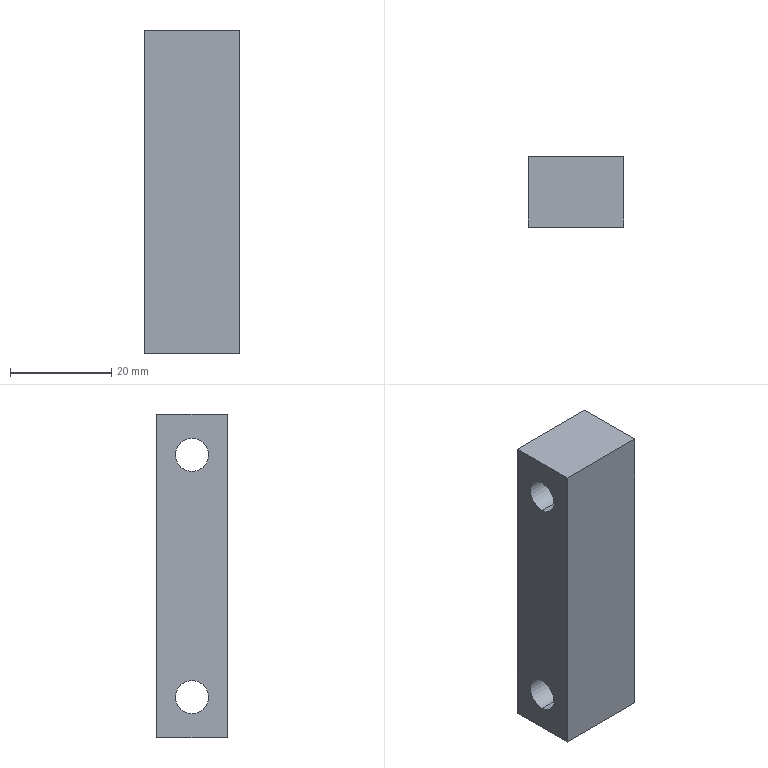Part | STEP file | 1 solid | 16 faces | box 19 x 14 x 64 mm | volume 14945 mm3 | cylinder 8 | plane 8 | commonest cylinder face diameters 6.6 x4 11 x4
STEP:
#1=CARTESIAN_POINT('',(0.,0.,0.));
#2=DIRECTION('',(0.,0.,1.));
#3=DIRECTION('',(1.,0.,0.));
#4=AXIS2_PLACEMENT_3D('',#1,#2,#3);
#5=CARTESIAN_POINT('',(12.6,0.,18.5));
#6=VERTEX_POINT('',#5);
#7=CARTESIAN_POINT('',(19.,0.,18.5));
#8=VERTEX_POINT('',#7);
#9=CARTESIAN_POINT('',(19.,0.,18.5));
#10=DIRECTION('',(1.,0.,0.));
#11=VECTOR('',#10,1.);
#12=LINE('',#9,#11);
#13=CARTESIAN_POINT('',(19.,0.,24.));
#14=DIRECTION('',(1.,0.,0.));
#15=DIRECTION('',(0.,0.,-1.));
#16=AXIS2_PLACEMENT_3D('',#13,#14,#15);
#17=CYLINDRICAL_SURFACE('',#16,5.5);
#18=CARTESIAN_POINT('',(6.283,0.));
#19=DIRECTION('',(0.,1.));
#20=VECTOR('',#19,1.);
#21=LINE('',#18,#20);
#22=(GEOMETRIC_REPRESENTATION_CONTEXT(2)PARAMETRIC_REPRESENTATION_CONTEXT()REPRESENTATION_CONTEXT('',''));
#23=DEFINITIONAL_REPRESENTATION('',(#21),#22);
#24=PCURVE('',#17,#23);
#25=CARTESIAN_POINT('',(19.,0.,24.));
#26=DIRECTION('',(1.,0.,0.));
#27=DIRECTION('',(0.,0.,-1.));
#28=AXIS2_PLACEMENT_3D('',#25,#26,#27);
#29=CYLINDRICAL_SURFACE('',#28,5.5);
#30=CARTESIAN_POINT('',(0.,0.));
#31=DIRECTION('',(0.,1.));
#32=VECTOR('',#31,1.);
#33=LINE('',#30,#32);
#34=(GEOMETRIC_REPRESENTATION_CONTEXT(2)PARAMETRIC_REPRESENTATION_CONTEXT()REPRESENTATION_CONTEXT('',''));
#35=DEFINITIONAL_REPRESENTATION('',(#33),#34);
#36=PCURVE('',#29,#35);
#37=SURFACE_CURVE('',#12,(#24,#36),.PCURVE_S1.);
#38=EDGE_CURVE('',#6,#8,#37,.T.);
#39=ORIENTED_EDGE('',*,*,#38,.T.);
#40=CARTESIAN_POINT('',(19.,0.,29.5));
#41=VERTEX_POINT('',#40);
#42=CARTESIAN_POINT('',(19.,0.,24.));
#43=DIRECTION('',(1.,0.,0.));
#44=DIRECTION('',(0.,0.,-1.));
#45=AXIS2_PLACEMENT_3D('',#42,#43,#44);
#46=CIRCLE('',#45,5.5);
#47=CARTESIAN_POINT('',(0.,0.));
#48=DIRECTION('',(1.,0.));
#49=VECTOR('',#48,1.);
#50=LINE('',#47,#49);
#51=(GEOMETRIC_REPRESENTATION_CONTEXT(2)PARAMETRIC_REPRESENTATION_CONTEXT()REPRESENTATION_CONTEXT('',''));
#52=DEFINITIONAL_REPRESENTATION('',(#50),#51);
#53=PCURVE('',#17,#52);
#54=CARTESIAN_POINT('',(19.,0.,0.));
#55=DIRECTION('',(1.,0.,0.));
#56=DIRECTION('',(0.,0.,-1.));
#57=AXIS2_PLACEMENT_3D('',#54,#55,#56);
#58=PLANE('',#57);
#59=CARTESIAN_POINT('',(-24.,0.));
#60=DIRECTION('',(1.,0.));
#61=AXIS2_PLACEMENT_2D('',#59,#60);
#62=CIRCLE('',#61,5.5);
#63=(GEOMETRIC_REPRESENTATION_CONTEXT(2)PARAMETRIC_REPRESENTATION_CONTEXT()REPRESENTATION_CONTEXT('',''));
#64=DEFINITIONAL_REPRESENTATION('',(#62),#63);
#65=PCURVE('',#58,#64);
#66=SURFACE_CURVE('',#46,(#53,#65),.PCURVE_S1.);
#67=EDGE_CURVE('',#41,#8,#66,.T.);
#68=ORIENTED_EDGE('',*,*,#67,.F.);
#69=CARTESIAN_POINT('',(12.6,0.,29.5));
#70=VERTEX_POINT('',#69);
#71=CARTESIAN_POINT('',(19.,0.,29.5));
#72=DIRECTION('',(1.,0.,0.));
#73=VECTOR('',#72,1.);
#74=LINE('',#71,#73);
#75=CARTESIAN_POINT('',(3.142,0.));
#76=DIRECTION('',(0.,1.));
#77=VECTOR('',#76,1.);
#78=LINE('',#75,#77);
#79=(GEOMETRIC_REPRESENTATION_CONTEXT(2)PARAMETRIC_REPRESENTATION_CONTEXT()REPRESENTATION_CONTEXT('',''));
#80=DEFINITIONAL_REPRESENTATION('',(#78),#79);
#81=PCURVE('',#17,#80);
#82=CARTESIAN_POINT('',(3.142,0.));
#83=DIRECTION('',(0.,1.));
#84=VECTOR('',#83,1.);
#85=LINE('',#82,#84);
#86=(GEOMETRIC_REPRESENTATION_CONTEXT(2)PARAMETRIC_REPRESENTATION_CONTEXT()REPRESENTATION_CONTEXT('',''));
#87=DEFINITIONAL_REPRESENTATION('',(#85),#86);
#88=PCURVE('',#29,#87);
#89=SURFACE_CURVE('',#74,(#81,#88),.PCURVE_S1.);
#90=EDGE_CURVE('',#70,#41,#89,.T.);
#91=ORIENTED_EDGE('',*,*,#90,.F.);
#92=CARTESIAN_POINT('',(12.6,0.,24.));
#93=DIRECTION('',(1.,0.,0.));
#94=DIRECTION('',(0.,0.,-1.));
#95=AXIS2_PLACEMENT_3D('',#92,#93,#94);
#96=CIRCLE('',#95,5.5);
#97=CARTESIAN_POINT('',(0.,-6.4));
#98=DIRECTION('',(1.,0.));
#99=VECTOR('',#98,1.);
#100=LINE('',#97,#99);
#101=(GEOMETRIC_REPRESENTATION_CONTEXT(2)PARAMETRIC_REPRESENTATION_CONTEXT()REPRESENTATION_CONTEXT('',''));
#102=DEFINITIONAL_REPRESENTATION('',(#100),#101);
#103=PCURVE('',#17,#102);
#104=CARTESIAN_POINT('',(12.6,3.3,24.));
#105=DIRECTION('',(-1.,0.,0.));
#106=DIRECTION('',(0.,0.,1.));
#107=AXIS2_PLACEMENT_3D('',#104,#105,#106);
#108=PLANE('',#107);
#109=CARTESIAN_POINT('',(-5.5,-3.3));
#110=CARTESIAN_POINT('',(-5.5,6.226));
#111=CARTESIAN_POINT('',(2.75,1.463));
#112=CARTESIAN_POINT('',(11.,-3.3));
#113=CARTESIAN_POINT('',(2.75,-8.063));
#114=CARTESIAN_POINT('',(-5.5,-12.826));
#115=CARTESIAN_POINT('',(-5.5,-3.3));
#116=(BOUNDED_CURVE()B_SPLINE_CURVE(2,(#109,#110,#111,#112,#113,#114,#115),.UNSPECIFIED.,.T.,.F.)B_SPLINE_CURVE_WITH_KNOTS((1,2,2,2,2,1),(-2.094,0.,2.094,4.189,6.283,8.378),.UNSPECIFIED.)CURVE()GEOMETRIC_REPRESENTATION_ITEM()RATIONAL_B_SPLINE_CURVE((1.,0.5,1.,0.5,1.,0.5,1.))REPRESENTATION_ITEM(''));
#117=(GEOMETRIC_REPRESENTATION_CONTEXT(2)PARAMETRIC_REPRESENTATION_CONTEXT()REPRESENTATION_CONTEXT('',''));
#118=DEFINITIONAL_REPRESENTATION('',(#116),#117);
#119=PCURVE('',#108,#118);
#120=SURFACE_CURVE('',#96,(#103,#119),.PCURVE_S1.);
#121=EDGE_CURVE('',#70,#6,#120,.T.);
#122=ORIENTED_EDGE('',*,*,#121,.T.);
#123=EDGE_LOOP('',(#39,#68,#91,#122));
#124=FACE_BOUND('',#123,.F.);
#125=ADVANCED_FACE('',(#124),#17,.F.);
#126=CARTESIAN_POINT('',(0.,0.,20.7));
#127=VERTEX_POINT('',#126);
#128=CARTESIAN_POINT('',(12.6,0.,20.7));
#129=VERTEX_POINT('',#128);
#130=CARTESIAN_POINT('',(19.,0.,20.7));
#131=DIRECTION('',(1.,0.,0.));
#132=VECTOR('',#131,1.);
#133=LINE('',#130,#132);
#134=CARTESIAN_POINT('',(19.,0.,24.));
#135=DIRECTION('',(1.,0.,0.));
#136=DIRECTION('',(0.,0.,-1.));
#137=AXIS2_PLACEMENT_3D('',#134,#135,#136);
#138=CYLINDRICAL_SURFACE('',#137,3.3);
#139=CARTESIAN_POINT('',(6.283,0.));
#140=DIRECTION('',(0.,1.));
#141=VECTOR('',#140,1.);
#142=LINE('',#139,#141);
#143=(GEOMETRIC_REPRESENTATION_CONTEXT(2)PARAMETRIC_REPRESENTATION_CONTEXT()REPRESENTATION_CONTEXT('',''));
#144=DEFINITIONAL_REPRESENTATION('',(#142),#143);
#145=PCURVE('',#138,#144);
#146=CARTESIAN_POINT('',(19.,0.,24.));
#147=DIRECTION('',(1.,0.,0.));
#148=DIRECTION('',(0.,0.,-1.));
#149=AXIS2_PLACEMENT_3D('',#146,#147,#148);
#150=CYLINDRICAL_SURFACE('',#149,3.3);
#151=CARTESIAN_POINT('',(0.,0.));
#152=DIRECTION('',(0.,1.));
#153=VECTOR('',#152,1.);
#154=LINE('',#151,#153);
#155=(GEOMETRIC_REPRESENTATION_CONTEXT(2)PARAMETRIC_REPRESENTATION_CONTEXT()REPRESENTATION_CONTEXT('',''));
#156=DEFINITIONAL_REPRESENTATION('',(#154),#155);
#157=PCURVE('',#150,#156);
#158=SURFACE_CURVE('',#133,(#145,#157),.PCURVE_S1.);
#159=EDGE_CURVE('',#127,#129,#158,.T.);
#160=ORIENTED_EDGE('',*,*,#159,.T.);
#161=CARTESIAN_POINT('',(12.6,0.,27.3));
#162=VERTEX_POINT('',#161);
#163=CARTESIAN_POINT('',(12.6,0.,24.));
#164=DIRECTION('',(1.,0.,0.));
#165=DIRECTION('',(0.,0.,-1.));
#166=AXIS2_PLACEMENT_3D('',#163,#164,#165);
#167=CIRCLE('',#166,3.3);
#168=CARTESIAN_POINT('',(0.,-6.4));
#169=DIRECTION('',(1.,0.));
#170=VECTOR('',#169,1.);
#171=LINE('',#168,#170);
#172=(GEOMETRIC_REPRESENTATION_CONTEXT(2)PARAMETRIC_REPRESENTATION_CONTEXT()REPRESENTATION_CONTEXT('',''));
#173=DEFINITIONAL_REPRESENTATION('',(#171),#172);
#174=PCURVE('',#138,#173);
#175=CARTESIAN_POINT('',(-3.3,-3.3));
#176=CARTESIAN_POINT('',(-3.3,2.416));
#177=CARTESIAN_POINT('',(1.65,-0.4421));
#178=CARTESIAN_POINT('',(6.6,-3.3));
#179=CARTESIAN_POINT('',(1.65,-6.158));
#180=CARTESIAN_POINT('',(-3.3,-9.016));
#181=CARTESIAN_POINT('',(-3.3,-3.3));
#182=(BOUNDED_CURVE()B_SPLINE_CURVE(2,(#175,#176,#177,#178,#179,#180,#181),.UNSPECIFIED.,.T.,.F.)B_SPLINE_CURVE_WITH_KNOTS((1,2,2,2,2,1),(-2.094,0.,2.094,4.189,6.283,8.378),.UNSPECIFIED.)CURVE()GEOMETRIC_REPRESENTATION_ITEM()RATIONAL_B_SPLINE_CURVE((1.,0.5,1.,0.5,1.,0.5,1.))REPRESENTATION_ITEM(''));
#183=(GEOMETRIC_REPRESENTATION_CONTEXT(2)PARAMETRIC_REPRESENTATION_CONTEXT()REPRESENTATION_CONTEXT('',''));
#184=DEFINITIONAL_REPRESENTATION('',(#182),#183);
#185=PCURVE('',#108,#184);
#186=SURFACE_CURVE('',#167,(#174,#185),.PCURVE_S1.);
#187=EDGE_CURVE('',#162,#129,#186,.T.);
#188=ORIENTED_EDGE('',*,*,#187,.F.);
#189=CARTESIAN_POINT('',(0.,0.,27.3));
#190=VERTEX_POINT('',#189);
#191=CARTESIAN_POINT('',(19.,0.,27.3));
#192=DIRECTION('',(1.,0.,0.));
#193=VECTOR('',#192,1.);
#194=LINE('',#191,#193);
#195=CARTESIAN_POINT('',(3.142,0.));
#196=DIRECTION('',(0.,1.));
#197=VECTOR('',#196,1.);
#198=LINE('',#195,#197);
#199=(GEOMETRIC_REPRESENTATION_CONTEXT(2)PARAMETRIC_REPRESENTATION_CONTEXT()REPRESENTATION_CONTEXT('',''));
#200=DEFINITIONAL_REPRESENTATION('',(#198),#199);
#201=PCURVE('',#138,#200);
#202=CARTESIAN_POINT('',(3.142,0.));
#203=DIRECTION('',(0.,1.));
#204=VECTOR('',#203,1.);
#205=LINE('',#202,#204);
#206=(GEOMETRIC_REPRESENTATION_CONTEXT(2)PARAMETRIC_REPRESENTATION_CONTEXT()REPRESENTATION_CONTEXT('',''));
#207=DEFINITIONAL_REPRESENTATION('',(#205),#206);
#208=PCURVE('',#150,#207);
#209=SURFACE_CURVE('',#194,(#201,#208),.PCURVE_S1.);
#210=EDGE_CURVE('',#190,#162,#209,.T.);
#211=ORIENTED_EDGE('',*,*,#210,.F.);
#212=CARTESIAN_POINT('',(0.,0.,24.));
#213=DIRECTION('',(1.,0.,0.));
#214=DIRECTION('',(0.,0.,-1.));
#215=AXIS2_PLACEMENT_3D('',#212,#213,#214);
#216=CIRCLE('',#215,3.3);
#217=CARTESIAN_POINT('',(0.,-19.));
#218=DIRECTION('',(1.,0.));
#219=VECTOR('',#218,1.);
#220=LINE('',#217,#219);
#221=(GEOMETRIC_REPRESENTATION_CONTEXT(2)PARAMETRIC_REPRESENTATION_CONTEXT()REPRESENTATION_CONTEXT('',''));
#222=DEFINITIONAL_REPRESENTATION('',(#220),#221);
#223=PCURVE('',#138,#222);
#224=CARTESIAN_POINT('',(0.,0.,0.));
#225=DIRECTION('',(1.,0.,0.));
#226=DIRECTION('',(0.,0.,-1.));
#227=AXIS2_PLACEMENT_3D('',#224,#225,#226);
#228=PLANE('',#227);
#229=CARTESIAN_POINT('',(-24.,0.));
#230=DIRECTION('',(1.,0.));
#231=AXIS2_PLACEMENT_2D('',#229,#230);
#232=CIRCLE('',#231,3.3);
#233=(GEOMETRIC_REPRESENTATION_CONTEXT(2)PARAMETRIC_REPRESENTATION_CONTEXT()REPRESENTATION_CONTEXT('',''));
#234=DEFINITIONAL_REPRESENTATION('',(#232),#233);
#235=PCURVE('',#228,#234);
#236=SURFACE_CURVE('',#216,(#223,#235),.PCURVE_S1.);
#237=EDGE_CURVE('',#190,#127,#236,.T.);
#238=ORIENTED_EDGE('',*,*,#237,.T.);
#239=EDGE_LOOP('',(#160,#188,#211,#238));
#240=FACE_BOUND('',#239,.F.);
#241=ADVANCED_FACE('',(#240),#138,.F.);
#242=CARTESIAN_POINT('',(12.6,0.,-29.5));
#243=VERTEX_POINT('',#242);
#244=CARTESIAN_POINT('',(19.,0.,-29.5));
#245=VERTEX_POINT('',#244);
#246=CARTESIAN_POINT('',(19.,0.,-29.5));
#247=DIRECTION('',(1.,0.,0.));
#248=VECTOR('',#247,1.);
#249=LINE('',#246,#248);
#250=CARTESIAN_POINT('',(19.,0.,-24.));
#251=DIRECTION('',(1.,0.,0.));
#252=DIRECTION('',(0.,0.,-1.));
#253=AXIS2_PLACEMENT_3D('',#250,#251,#252);
#254=CYLINDRICAL_SURFACE('',#253,5.5);
#255=CARTESIAN_POINT('',(6.283,0.));
#256=DIRECTION('',(0.,1.));
#257=VECTOR('',#256,1.);
#258=LINE('',#255,#257);
#259=(GEOMETRIC_REPRESENTATION_CONTEXT(2)PARAMETRIC_REPRESENTATION_CONTEXT()REPRESENTATION_CONTEXT('',''));
#260=DEFINITIONAL_REPRESENTATION('',(#258),#259);
#261=PCURVE('',#254,#260);
#262=CARTESIAN_POINT('',(19.,0.,-24.));
#263=DIRECTION('',(1.,0.,0.));
#264=DIRECTION('',(0.,0.,-1.));
#265=AXIS2_PLACEMENT_3D('',#262,#263,#264);
#266=CYLINDRICAL_SURFACE('',#265,5.5);
#267=CARTESIAN_POINT('',(0.,0.));
#268=DIRECTION('',(0.,1.));
#269=VECTOR('',#268,1.);
#270=LINE('',#267,#269);
#271=(GEOMETRIC_REPRESENTATION_CONTEXT(2)PARAMETRIC_REPRESENTATION_CONTEXT()REPRESENTATION_CONTEXT('',''));
#272=DEFINITIONAL_REPRESENTATION('',(#270),#271);
#273=PCURVE('',#266,#272);
#274=SURFACE_CURVE('',#249,(#261,#273),.PCURVE_S1.);
#275=EDGE_CURVE('',#243,#245,#274,.T.);
#276=ORIENTED_EDGE('',*,*,#275,.T.);
#277=CARTESIAN_POINT('',(19.,0.,-18.5));
#278=VERTEX_POINT('',#277);
#279=CARTESIAN_POINT('',(19.,0.,-24.));
#280=DIRECTION('',(1.,0.,0.));
#281=DIRECTION('',(0.,0.,-1.));
#282=AXIS2_PLACEMENT_3D('',#279,#280,#281);
#283=CIRCLE('',#282,5.5);
#284=CARTESIAN_POINT('',(0.,0.));
#285=DIRECTION('',(1.,0.));
#286=VECTOR('',#285,1.);
#287=LINE('',#284,#286);
#288=(GEOMETRIC_REPRESENTATION_CONTEXT(2)PARAMETRIC_REPRESENTATION_CONTEXT()REPRESENTATION_CONTEXT('',''));
#289=DEFINITIONAL_REPRESENTATION('',(#287),#288);
#290=PCURVE('',#254,#289);
#291=CARTESIAN_POINT('',(24.,0.));
#292=DIRECTION('',(1.,0.));
#293=AXIS2_PLACEMENT_2D('',#291,#292);
#294=CIRCLE('',#293,5.5);
#295=(GEOMETRIC_REPRESENTATION_CONTEXT(2)PARAMETRIC_REPRESENTATION_CONTEXT()REPRESENTATION_CONTEXT('',''));
#296=DEFINITIONAL_REPRESENTATION('',(#294),#295);
#297=PCURVE('',#58,#296);
#298=SURFACE_CURVE('',#283,(#290,#297),.PCURVE_S1.);
#299=EDGE_CURVE('',#278,#245,#298,.T.);
#300=ORIENTED_EDGE('',*,*,#299,.F.);
#301=CARTESIAN_POINT('',(12.6,0.,-18.5));
#302=VERTEX_POINT('',#301);
#303=CARTESIAN_POINT('',(19.,0.,-18.5));
#304=DIRECTION('',(1.,0.,0.));
#305=VECTOR('',#304,1.);
#306=LINE('',#303,#305);
#307=CARTESIAN_POINT('',(3.142,0.));
#308=DIRECTION('',(0.,1.));
#309=VECTOR('',#308,1.);
#310=LINE('',#307,#309);
#311=(GEOMETRIC_REPRESENTATION_CONTEXT(2)PARAMETRIC_REPRESENTATION_CONTEXT()REPRESENTATION_CONTEXT('',''));
#312=DEFINITIONAL_REPRESENTATION('',(#310),#311);
#313=PCURVE('',#254,#312);
#314=CARTESIAN_POINT('',(3.142,0.));
#315=DIRECTION('',(0.,1.));
#316=VECTOR('',#315,1.);
#317=LINE('',#314,#316);
#318=(GEOMETRIC_REPRESENTATION_CONTEXT(2)PARAMETRIC_REPRESENTATION_CONTEXT()REPRESENTATION_CONTEXT('',''));
#319=DEFINITIONAL_REPRESENTATION('',(#317),#318);
#320=PCURVE('',#266,#319);
#321=SURFACE_CURVE('',#306,(#313,#320),.PCURVE_S1.);
#322=EDGE_CURVE('',#302,#278,#321,.T.);
#323=ORIENTED_EDGE('',*,*,#322,.F.);
#324=CARTESIAN_POINT('',(12.6,0.,-24.));
#325=DIRECTION('',(1.,0.,0.));
#326=DIRECTION('',(0.,0.,-1.));
#327=AXIS2_PLACEMENT_3D('',#324,#325,#326);
#328=CIRCLE('',#327,5.5);
#329=CARTESIAN_POINT('',(0.,-6.4));
#330=DIRECTION('',(1.,0.));
#331=VECTOR('',#330,1.);
#332=LINE('',#329,#331);
#333=(GEOMETRIC_REPRESENTATION_CONTEXT(2)PARAMETRIC_REPRESENTATION_CONTEXT()REPRESENTATION_CONTEXT('',''));
#334=DEFINITIONAL_REPRESENTATION('',(#332),#333);
#335=PCURVE('',#254,#334);
#336=CARTESIAN_POINT('',(12.6,3.3,-24.));
#337=DIRECTION('',(-1.,0.,0.));
#338=DIRECTION('',(0.,0.,1.));
#339=AXIS2_PLACEMENT_3D('',#336,#337,#338);
#340=PLANE('',#339);
#341=CARTESIAN_POINT('',(-5.5,-3.3));
#342=CARTESIAN_POINT('',(-5.5,6.226));
#343=CARTESIAN_POINT('',(2.75,1.463));
#344=CARTESIAN_POINT('',(11.,-3.3));
#345=CARTESIAN_POINT('',(2.75,-8.063));
#346=CARTESIAN_POINT('',(-5.5,-12.826));
#347=CARTESIAN_POINT('',(-5.5,-3.3));
#348=(BOUNDED_CURVE()B_SPLINE_CURVE(2,(#341,#342,#343,#344,#345,#346,#347),.UNSPECIFIED.,.T.,.F.)B_SPLINE_CURVE_WITH_KNOTS((1,2,2,2,2,1),(-2.094,0.,2.094,4.189,6.283,8.378),.UNSPECIFIED.)CURVE()GEOMETRIC_REPRESENTATION_ITEM()RATIONAL_B_SPLINE_CURVE((1.,0.5,1.,0.5,1.,0.5,1.))REPRESENTATION_ITEM(''));
#349=(GEOMETRIC_REPRESENTATION_CONTEXT(2)PARAMETRIC_REPRESENTATION_CONTEXT()REPRESENTATION_CONTEXT('',''));
#350=DEFINITIONAL_REPRESENTATION('',(#348),#349);
#351=PCURVE('',#340,#350);
#352=SURFACE_CURVE('',#328,(#335,#351),.PCURVE_S1.);
#353=EDGE_CURVE('',#302,#243,#352,.T.);
#354=ORIENTED_EDGE('',*,*,#353,.T.);
#355=EDGE_LOOP('',(#276,#300,#323,#354));
#356=FACE_BOUND('',#355,.F.);
#357=ADVANCED_FACE('',(#356),#254,.F.);
#358=CARTESIAN_POINT('',(0.,0.,-27.3));
#359=VERTEX_POINT('',#358);
#360=CARTESIAN_POINT('',(12.6,0.,-27.3));
#361=VERTEX_POINT('',#360);
#362=CARTESIAN_POINT('',(19.,0.,-27.3));
#363=DIRECTION('',(1.,0.,0.));
#364=VECTOR('',#363,1.);
#365=LINE('',#362,#364);
#366=CARTESIAN_POINT('',(19.,0.,-24.));
#367=DIRECTION('',(1.,0.,0.));
#368=DIRECTION('',(0.,0.,-1.));
#369=AXIS2_PLACEMENT_3D('',#366,#367,#368);
#370=CYLINDRICAL_SURFACE('',#369,3.3);
#371=CARTESIAN_POINT('',(6.283,0.));
#372=DIRECTION('',(0.,1.));
#373=VECTOR('',#372,1.);
#374=LINE('',#371,#373);
#375=(GEOMETRIC_REPRESENTATION_CONTEXT(2)PARAMETRIC_REPRESENTATION_CONTEXT()REPRESENTATION_CONTEXT('',''));
#376=DEFINITIONAL_REPRESENTATION('',(#374),#375);
#377=PCURVE('',#370,#376);
#378=CARTESIAN_POINT('',(19.,0.,-24.));
#379=DIRECTION('',(1.,0.,0.));
#380=DIRECTION('',(0.,0.,-1.));
#381=AXIS2_PLACEMENT_3D('',#378,#379,#380);
#382=CYLINDRICAL_SURFACE('',#381,3.3);
#383=CARTESIAN_POINT('',(0.,0.));
#384=DIRECTION('',(0.,1.));
#385=VECTOR('',#384,1.);
#386=LINE('',#383,#385);
#387=(GEOMETRIC_REPRESENTATION_CONTEXT(2)PARAMETRIC_REPRESENTATION_CONTEXT()REPRESENTATION_CONTEXT('',''));
#388=DEFINITIONAL_REPRESENTATION('',(#386),#387);
#389=PCURVE('',#382,#388);
#390=SURFACE_CURVE('',#365,(#377,#389),.PCURVE_S1.);
#391=EDGE_CURVE('',#359,#361,#390,.T.);
#392=ORIENTED_EDGE('',*,*,#391,.T.);
#393=CARTESIAN_POINT('',(12.6,0.,-20.7));
#394=VERTEX_POINT('',#393);
#395=CARTESIAN_POINT('',(12.6,0.,-24.));
#396=DIRECTION('',(1.,0.,0.));
#397=DIRECTION('',(0.,0.,-1.));
#398=AXIS2_PLACEMENT_3D('',#395,#396,#397);
#399=CIRCLE('',#398,3.3);
#400=CARTESIAN_POINT('',(0.,-6.4));
#401=DIRECTION('',(1.,0.));
#402=VECTOR('',#401,1.);
#403=LINE('',#400,#402);
#404=(GEOMETRIC_REPRESENTATION_CONTEXT(2)PARAMETRIC_REPRESENTATION_CONTEXT()REPRESENTATION_CONTEXT('',''));
#405=DEFINITIONAL_REPRESENTATION('',(#403),#404);
#406=PCURVE('',#370,#405);
#407=CARTESIAN_POINT('',(-3.3,-3.3));
#408=CARTESIAN_POINT('',(-3.3,2.416));
#409=CARTESIAN_POINT('',(1.65,-0.4421));
#410=CARTESIAN_POINT('',(6.6,-3.3));
#411=CARTESIAN_POINT('',(1.65,-6.158));
#412=CARTESIAN_POINT('',(-3.3,-9.016));
#413=CARTESIAN_POINT('',(-3.3,-3.3));
#414=(BOUNDED_CURVE()B_SPLINE_CURVE(2,(#407,#408,#409,#410,#411,#412,#413),.UNSPECIFIED.,.T.,.F.)B_SPLINE_CURVE_WITH_KNOTS((1,2,2,2,2,1),(-2.094,0.,2.094,4.189,6.283,8.378),.UNSPECIFIED.)CURVE()GEOMETRIC_REPRESENTATION_ITEM()RATIONAL_B_SPLINE_CURVE((1.,0.5,1.,0.5,1.,0.5,1.))REPRESENTATION_ITEM(''));
#415=(GEOMETRIC_REPRESENTATION_CONTEXT(2)PARAMETRIC_REPRESENTATION_CONTEXT()REPRESENTATION_CONTEXT('',''));
#416=DEFINITIONAL_REPRESENTATION('',(#414),#415);
#417=PCURVE('',#340,#416);
#418=SURFACE_CURVE('',#399,(#406,#417),.PCURVE_S1.);
#419=EDGE_CURVE('',#394,#361,#418,.T.);
#420=ORIENTED_EDGE('',*,*,#419,.F.);
#421=CARTESIAN_POINT('',(0.,0.,-20.7));
#422=VERTEX_POINT('',#421);
#423=CARTESIAN_POINT('',(19.,0.,-20.7));
#424=DIRECTION('',(1.,0.,0.));
#425=VECTOR('',#424,1.);
#426=LINE('',#423,#425);
#427=CARTESIAN_POINT('',(3.142,0.));
#428=DIRECTION('',(0.,1.));
#429=VECTOR('',#428,1.);
#430=LINE('',#427,#429);
#431=(GEOMETRIC_REPRESENTATION_CONTEXT(2)PARAMETRIC_REPRESENTATION_CONTEXT()REPRESENTATION_CONTEXT('',''));
#432=DEFINITIONAL_REPRESENTATION('',(#430),#431);
#433=PCURVE('',#370,#432);
#434=CARTESIAN_POINT('',(3.142,0.));
#435=DIRECTION('',(0.,1.));
#436=VECTOR('',#435,1.);
#437=LINE('',#434,#436);
#438=(GEOMETRIC_REPRESENTATION_CONTEXT(2)PARAMETRIC_REPRESENTATION_CONTEXT()REPRESENTATION_CONTEXT('',''));
#439=DEFINITIONAL_REPRESENTATION('',(#437),#438);
#440=PCURVE('',#382,#439);
#441=SURFACE_CURVE('',#426,(#433,#440),.PCURVE_S1.);
#442=EDGE_CURVE('',#422,#394,#441,.T.);
#443=ORIENTED_EDGE('',*,*,#442,.F.);
#444=CARTESIAN_POINT('',(0.,0.,-24.));
#445=DIRECTION('',(1.,0.,0.));
#446=DIRECTION('',(0.,0.,-1.));
#447=AXIS2_PLACEMENT_3D('',#444,#445,#446);
#448=CIRCLE('',#447,3.3);
#449=CARTESIAN_POINT('',(0.,-19.));
#450=DIRECTION('',(1.,0.));
#451=VECTOR('',#450,1.);
#452=LINE('',#449,#451);
#453=(GEOMETRIC_REPRESENTATION_CONTEXT(2)PARAMETRIC_REPRESENTATION_CONTEXT()REPRESENTATION_CONTEXT('',''));
#454=DEFINITIONAL_REPRESENTATION('',(#452),#453);
#455=PCURVE('',#370,#454);
#456=CARTESIAN_POINT('',(24.,0.));
#457=DIRECTION('',(1.,0.));
#458=AXIS2_PLACEMENT_2D('',#456,#457);
#459=CIRCLE('',#458,3.3);
#460=(GEOMETRIC_REPRESENTATION_CONTEXT(2)PARAMETRIC_REPRESENTATION_CONTEXT()REPRESENTATION_CONTEXT('',''));
#461=DEFINITIONAL_REPRESENTATION('',(#459),#460);
#462=PCURVE('',#228,#461);
#463=SURFACE_CURVE('',#448,(#455,#462),.PCURVE_S1.);
#464=EDGE_CURVE('',#422,#359,#463,.T.);
#465=ORIENTED_EDGE('',*,*,#464,.T.);
#466=EDGE_LOOP('',(#392,#420,#443,#465));
#467=FACE_BOUND('',#466,.F.);
#468=ADVANCED_FACE('',(#467),#370,.F.);
#469=CARTESIAN_POINT('',(0.,7.,32.));
#470=VERTEX_POINT('',#469);
#471=CARTESIAN_POINT('',(0.,-7.,32.));
#472=VERTEX_POINT('',#471);
#473=CARTESIAN_POINT('',(0.,-7.,32.));
#474=DIRECTION('',(0.,-1.,0.));
#475=VECTOR('',#474,1.);
#476=LINE('',#473,#475);
#477=CARTESIAN_POINT('',(19.,-7.,32.));
#478=DIRECTION('',(0.,0.,-1.));
#479=DIRECTION('',(-1.,0.,0.));
#480=AXIS2_PLACEMENT_3D('',#477,#478,#479);
#481=PLANE('',#480);
#482=CARTESIAN_POINT('',(19.,0.));
#483=DIRECTION('',(0.,-1.));
#484=VECTOR('',#483,1.);
#485=LINE('',#482,#484);
#486=(GEOMETRIC_REPRESENTATION_CONTEXT(2)PARAMETRIC_REPRESENTATION_CONTEXT()REPRESENTATION_CONTEXT('',''));
#487=DEFINITIONAL_REPRESENTATION('',(#485),#486);
#488=PCURVE('',#481,#487);
#489=CARTESIAN_POINT('',(-32.,-7.));
#490=DIRECTION('',(0.,-1.));
#491=VECTOR('',#490,1.);
#492=LINE('',#489,#491);
#493=(GEOMETRIC_REPRESENTATION_CONTEXT(2)PARAMETRIC_REPRESENTATION_CONTEXT()REPRESENTATION_CONTEXT('',''));
#494=DEFINITIONAL_REPRESENTATION('',(#492),#493);
#495=PCURVE('',#228,#494);
#496=SURFACE_CURVE('',#476,(#488,#495),.PCURVE_S1.);
#497=EDGE_CURVE('',#470,#472,#496,.T.);
#498=ORIENTED_EDGE('',*,*,#497,.T.);
#499=CARTESIAN_POINT('',(19.,-7.,32.));
#500=VERTEX_POINT('',#499);
#501=CARTESIAN_POINT('',(19.,-7.,32.));
#502=DIRECTION('',(-1.,0.,0.));
#503=VECTOR('',#502,1.);
#504=LINE('',#501,#503);
#505=CARTESIAN_POINT('',(0.,0.));
#506=DIRECTION('',(1.,0.));
#507=VECTOR('',#506,1.);
#508=LINE('',#505,#507);
#509=(GEOMETRIC_REPRESENTATION_CONTEXT(2)PARAMETRIC_REPRESENTATION_CONTEXT()REPRESENTATION_CONTEXT('',''));
#510=DEFINITIONAL_REPRESENTATION('',(#508),#509);
#511=PCURVE('',#481,#510);
#512=CARTESIAN_POINT('',(19.,-7.,-32.));
#513=DIRECTION('',(0.,1.,0.));
#514=DIRECTION('',(0.,0.,1.));
#515=AXIS2_PLACEMENT_3D('',#512,#513,#514);
#516=PLANE('',#515);
#517=CARTESIAN_POINT('',(64.,0.));
#518=DIRECTION('',(0.,-1.));
#519=VECTOR('',#518,1.);
#520=LINE('',#517,#519);
#521=(GEOMETRIC_REPRESENTATION_CONTEXT(2)PARAMETRIC_REPRESENTATION_CONTEXT()REPRESENTATION_CONTEXT('',''));
#522=DEFINITIONAL_REPRESENTATION('',(#520),#521);
#523=PCURVE('',#516,#522);
#524=SURFACE_CURVE('',#504,(#511,#523),.PCURVE_S1.);
#525=EDGE_CURVE('',#500,#472,#524,.T.);
#526=ORIENTED_EDGE('',*,*,#525,.F.);
#527=CARTESIAN_POINT('',(19.,7.,32.));
#528=VERTEX_POINT('',#527);
#529=CARTESIAN_POINT('',(19.,-7.,32.));
#530=DIRECTION('',(0.,-1.,0.));
#531=VECTOR('',#530,1.);
#532=LINE('',#529,#531);
#533=CARTESIAN_POINT('',(0.,0.));
#534=DIRECTION('',(0.,-1.));
#535=VECTOR('',#534,1.);
#536=LINE('',#533,#535);
#537=(GEOMETRIC_REPRESENTATION_CONTEXT(2)PARAMETRIC_REPRESENTATION_CONTEXT()REPRESENTATION_CONTEXT('',''));
#538=DEFINITIONAL_REPRESENTATION('',(#536),#537);
#539=PCURVE('',#481,#538);
#540=CARTESIAN_POINT('',(-32.,-7.));
#541=DIRECTION('',(0.,-1.));
#542=VECTOR('',#541,1.);
#543=LINE('',#540,#542);
#544=(GEOMETRIC_REPRESENTATION_CONTEXT(2)PARAMETRIC_REPRESENTATION_CONTEXT()REPRESENTATION_CONTEXT('',''));
#545=DEFINITIONAL_REPRESENTATION('',(#543),#544);
#546=PCURVE('',#58,#545);
#547=SURFACE_CURVE('',#532,(#539,#546),.PCURVE_S1.);
#548=EDGE_CURVE('',#528,#500,#547,.T.);
#549=ORIENTED_EDGE('',*,*,#548,.F.);
#550=CARTESIAN_POINT('',(19.,7.,32.));
#551=DIRECTION('',(-1.,0.,0.));
#552=VECTOR('',#551,1.);
#553=LINE('',#550,#552);
#554=CARTESIAN_POINT('',(0.,14.));
#555=DIRECTION('',(1.,0.));
#556=VECTOR('',#555,1.);
#557=LINE('',#554,#556);
#558=(GEOMETRIC_REPRESENTATION_CONTEXT(2)PARAMETRIC_REPRESENTATION_CONTEXT()REPRESENTATION_CONTEXT('',''));
#559=DEFINITIONAL_REPRESENTATION('',(#557),#558);
#560=PCURVE('',#481,#559);
#561=CARTESIAN_POINT('',(19.,7.,-32.));
#562=DIRECTION('',(0.,-1.,0.));
#563=DIRECTION('',(0.,0.,-1.));
#564=AXIS2_PLACEMENT_3D('',#561,#562,#563);
#565=PLANE('',#564);
#566=CARTESIAN_POINT('',(-64.,0.));
#567=DIRECTION('',(0.,-1.));
#568=VECTOR('',#567,1.);
#569=LINE('',#566,#568);
#570=(GEOMETRIC_REPRESENTATION_CONTEXT(2)PARAMETRIC_REPRESENTATION_CONTEXT()REPRESENTATION_CONTEXT('',''));
#571=DEFINITIONAL_REPRESENTATION('',(#569),#570);
#572=PCURVE('',#565,#571);
#573=SURFACE_CURVE('',#553,(#560,#572),.PCURVE_S1.);
#574=EDGE_CURVE('',#528,#470,#573,.T.);
#575=ORIENTED_EDGE('',*,*,#574,.T.);
#576=EDGE_LOOP('',(#498,#526,#549,#575));
#577=FACE_BOUND('',#576,.T.);
#578=ADVANCED_FACE('',(#577),#481,.F.);
#579=CARTESIAN_POINT('',(0.,-7.,-32.));
#580=VERTEX_POINT('',#579);
#581=CARTESIAN_POINT('',(0.,-7.,-32.));
#582=DIRECTION('',(0.,0.,-1.));
#583=VECTOR('',#582,1.);
#584=LINE('',#581,#583);
#585=CARTESIAN_POINT('',(0.,-19.));
#586=DIRECTION('',(-1.,0.));
#587=VECTOR('',#586,1.);
#588=LINE('',#585,#587);
#589=(GEOMETRIC_REPRESENTATION_CONTEXT(2)PARAMETRIC_REPRESENTATION_CONTEXT()REPRESENTATION_CONTEXT('',''));
#590=DEFINITIONAL_REPRESENTATION('',(#588),#589);
#591=PCURVE('',#516,#590);
#592=CARTESIAN_POINT('',(32.,-7.));
#593=DIRECTION('',(1.,0.));
#594=VECTOR('',#593,1.);
#595=LINE('',#592,#594);
#596=(GEOMETRIC_REPRESENTATION_CONTEXT(2)PARAMETRIC_REPRESENTATION_CONTEXT()REPRESENTATION_CONTEXT('',''));
#597=DEFINITIONAL_REPRESENTATION('',(#595),#596);
#598=PCURVE('',#228,#597);
#599=SURFACE_CURVE('',#584,(#591,#598),.PCURVE_S1.);
#600=EDGE_CURVE('',#472,#580,#599,.T.);
#601=ORIENTED_EDGE('',*,*,#600,.T.);
#602=CARTESIAN_POINT('',(19.,-7.,-32.));
#603=VERTEX_POINT('',#602);
#604=CARTESIAN_POINT('',(19.,-7.,-32.));
#605=DIRECTION('',(-1.,0.,0.));
#606=VECTOR('',#605,1.);
#607=LINE('',#604,#606);
#608=CARTESIAN_POINT('',(0.,0.));
#609=DIRECTION('',(0.,-1.));
#610=VECTOR('',#609,1.);
#611=LINE('',#608,#610);
#612=(GEOMETRIC_REPRESENTATION_CONTEXT(2)PARAMETRIC_REPRESENTATION_CONTEXT()REPRESENTATION_CONTEXT('',''));
#613=DEFINITIONAL_REPRESENTATION('',(#611),#612);
#614=PCURVE('',#516,#613);
#615=CARTESIAN_POINT('',(19.,-7.,-32.));
#616=DIRECTION('',(0.,0.,1.));
#617=DIRECTION('',(1.,0.,0.));
#618=AXIS2_PLACEMENT_3D('',#615,#616,#617);
#619=PLANE('',#618);
#620=CARTESIAN_POINT('',(0.,0.));
#621=DIRECTION('',(-1.,0.));
#622=VECTOR('',#621,1.);
#623=LINE('',#620,#622);
#624=(GEOMETRIC_REPRESENTATION_CONTEXT(2)PARAMETRIC_REPRESENTATION_CONTEXT()REPRESENTATION_CONTEXT('',''));
#625=DEFINITIONAL_REPRESENTATION('',(#623),#624);
#626=PCURVE('',#619,#625);
#627=SURFACE_CURVE('',#607,(#614,#626),.PCURVE_S1.);
#628=EDGE_CURVE('',#603,#580,#627,.T.);
#629=ORIENTED_EDGE('',*,*,#628,.F.);
#630=CARTESIAN_POINT('',(19.,-7.,-32.));
#631=DIRECTION('',(0.,0.,-1.));
#632=VECTOR('',#631,1.);
#633=LINE('',#630,#632);
#634=CARTESIAN_POINT('',(0.,0.));
#635=DIRECTION('',(-1.,0.));
#636=VECTOR('',#635,1.);
#637=LINE('',#634,#636);
#638=(GEOMETRIC_REPRESENTATION_CONTEXT(2)PARAMETRIC_REPRESENTATION_CONTEXT()REPRESENTATION_CONTEXT('',''));
#639=DEFINITIONAL_REPRESENTATION('',(#637),#638);
#640=PCURVE('',#516,#639);
#641=CARTESIAN_POINT('',(32.,-7.));
#642=DIRECTION('',(1.,0.));
#643=VECTOR('',#642,1.);
#644=LINE('',#641,#643);
#645=(GEOMETRIC_REPRESENTATION_CONTEXT(2)PARAMETRIC_REPRESENTATION_CONTEXT()REPRESENTATION_CONTEXT('',''));
#646=DEFINITIONAL_REPRESENTATION('',(#644),#645);
#647=PCURVE('',#58,#646);
#648=SURFACE_CURVE('',#633,(#640,#647),.PCURVE_S1.);
#649=EDGE_CURVE('',#500,#603,#648,.T.);
#650=ORIENTED_EDGE('',*,*,#649,.F.);
#651=ORIENTED_EDGE('',*,*,#525,.T.);
#652=EDGE_LOOP('',(#601,#629,#650,#651));
#653=FACE_BOUND('',#652,.T.);
#654=ADVANCED_FACE('',(#653),#516,.F.);
#655=CARTESIAN_POINT('',(0.,7.,-32.));
#656=VERTEX_POINT('',#655);
#657=CARTESIAN_POINT('',(0.,-7.,-32.));
#658=DIRECTION('',(0.,1.,0.));
#659=VECTOR('',#658,1.);
#660=LINE('',#657,#659);
#661=CARTESIAN_POINT('',(-19.,0.));
#662=DIRECTION('',(0.,1.));
#663=VECTOR('',#662,1.);
#664=LINE('',#661,#663);
#665=(GEOMETRIC_REPRESENTATION_CONTEXT(2)PARAMETRIC_REPRESENTATION_CONTEXT()REPRESENTATION_CONTEXT('',''));
#666=DEFINITIONAL_REPRESENTATION('',(#664),#665);
#667=PCURVE('',#619,#666);
#668=CARTESIAN_POINT('',(32.,-7.));
#669=DIRECTION('',(0.,1.));
#670=VECTOR('',#669,1.);
#671=LINE('',#668,#670);
#672=(GEOMETRIC_REPRESENTATION_CONTEXT(2)PARAMETRIC_REPRESENTATION_CONTEXT()REPRESENTATION_CONTEXT('',''));
#673=DEFINITIONAL_REPRESENTATION('',(#671),#672);
#674=PCURVE('',#228,#673);
#675=SURFACE_CURVE('',#660,(#667,#674),.PCURVE_S1.);
#676=EDGE_CURVE('',#580,#656,#675,.T.);
#677=ORIENTED_EDGE('',*,*,#676,.T.);
#678=CARTESIAN_POINT('',(19.,7.,-32.));
#679=VERTEX_POINT('',#678);
#680=CARTESIAN_POINT('',(19.,7.,-32.));
#681=DIRECTION('',(-1.,0.,0.));
#682=VECTOR('',#681,1.);
#683=LINE('',#680,#682);
#684=CARTESIAN_POINT('',(0.,14.));
#685=DIRECTION('',(-1.,0.));
#686=VECTOR('',#685,1.);
#687=LINE('',#684,#686);
#688=(GEOMETRIC_REPRESENTATION_CONTEXT(2)PARAMETRIC_REPRESENTATION_CONTEXT()REPRESENTATION_CONTEXT('',''));
#689=DEFINITIONAL_REPRESENTATION('',(#687),#688);
#690=PCURVE('',#619,#689);
#691=CARTESIAN_POINT('',(0.,0.));
#692=DIRECTION('',(0.,-1.));
#693=VECTOR('',#692,1.);
#694=LINE('',#691,#693);
#695=(GEOMETRIC_REPRESENTATION_CONTEXT(2)PARAMETRIC_REPRESENTATION_CONTEXT()REPRESENTATION_CONTEXT('',''));
#696=DEFINITIONAL_REPRESENTATION('',(#694),#695);
#697=PCURVE('',#565,#696);
#698=SURFACE_CURVE('',#683,(#690,#697),.PCURVE_S1.);
#699=EDGE_CURVE('',#679,#656,#698,.T.);
#700=ORIENTED_EDGE('',*,*,#699,.F.);
#701=CARTESIAN_POINT('',(19.,-7.,-32.));
#702=DIRECTION('',(0.,1.,0.));
#703=VECTOR('',#702,1.);
#704=LINE('',#701,#703);
#705=CARTESIAN_POINT('',(0.,0.));
#706=DIRECTION('',(0.,1.));
#707=VECTOR('',#706,1.);
#708=LINE('',#705,#707);
#709=(GEOMETRIC_REPRESENTATION_CONTEXT(2)PARAMETRIC_REPRESENTATION_CONTEXT()REPRESENTATION_CONTEXT('',''));
#710=DEFINITIONAL_REPRESENTATION('',(#708),#709);
#711=PCURVE('',#619,#710);
#712=CARTESIAN_POINT('',(32.,-7.));
#713=DIRECTION('',(0.,1.));
#714=VECTOR('',#713,1.);
#715=LINE('',#712,#714);
#716=(GEOMETRIC_REPRESENTATION_CONTEXT(2)PARAMETRIC_REPRESENTATION_CONTEXT()REPRESENTATION_CONTEXT('',''));
#717=DEFINITIONAL_REPRESENTATION('',(#715),#716);
#718=PCURVE('',#58,#717);
#719=SURFACE_CURVE('',#704,(#711,#718),.PCURVE_S1.);
#720=EDGE_CURVE('',#603,#679,#719,.T.);
#721=ORIENTED_EDGE('',*,*,#720,.F.);
#722=ORIENTED_EDGE('',*,*,#628,.T.);
#723=EDGE_LOOP('',(#677,#700,#721,#722));
#724=FACE_BOUND('',#723,.T.);
#725=ADVANCED_FACE('',(#724),#619,.F.);
#726=CARTESIAN_POINT('',(0.,7.,-32.));
#727=DIRECTION('',(0.,0.,1.));
#728=VECTOR('',#727,1.);
#729=LINE('',#726,#728);
#730=CARTESIAN_POINT('',(0.,-19.));
#731=DIRECTION('',(-1.,0.));
#732=VECTOR('',#731,1.);
#733=LINE('',#730,#732);
#734=(GEOMETRIC_REPRESENTATION_CONTEXT(2)PARAMETRIC_REPRESENTATION_CONTEXT()REPRESENTATION_CONTEXT('',''));
#735=DEFINITIONAL_REPRESENTATION('',(#733),#734);
#736=PCURVE('',#565,#735);
#737=CARTESIAN_POINT('',(32.,7.));
#738=DIRECTION('',(-1.,0.));
#739=VECTOR('',#738,1.);
#740=LINE('',#737,#739);
#741=(GEOMETRIC_REPRESENTATION_CONTEXT(2)PARAMETRIC_REPRESENTATION_CONTEXT()REPRESENTATION_CONTEXT('',''));
#742=DEFINITIONAL_REPRESENTATION('',(#740),#741);
#743=PCURVE('',#228,#742);
#744=SURFACE_CURVE('',#729,(#736,#743),.PCURVE_S1.);
#745=EDGE_CURVE('',#656,#470,#744,.T.);
#746=ORIENTED_EDGE('',*,*,#745,.T.);
#747=ORIENTED_EDGE('',*,*,#574,.F.);
#748=CARTESIAN_POINT('',(19.,7.,-32.));
#749=DIRECTION('',(0.,0.,1.));
#750=VECTOR('',#749,1.);
#751=LINE('',#748,#750);
#752=CARTESIAN_POINT('',(0.,0.));
#753=DIRECTION('',(-1.,0.));
#754=VECTOR('',#753,1.);
#755=LINE('',#752,#754);
#756=(GEOMETRIC_REPRESENTATION_CONTEXT(2)PARAMETRIC_REPRESENTATION_CONTEXT()REPRESENTATION_CONTEXT('',''));
#757=DEFINITIONAL_REPRESENTATION('',(#755),#756);
#758=PCURVE('',#565,#757);
#759=CARTESIAN_POINT('',(32.,7.));
#760=DIRECTION('',(-1.,0.));
#761=VECTOR('',#760,1.);
#762=LINE('',#759,#761);
#763=(GEOMETRIC_REPRESENTATION_CONTEXT(2)PARAMETRIC_REPRESENTATION_CONTEXT()REPRESENTATION_CONTEXT('',''));
#764=DEFINITIONAL_REPRESENTATION('',(#762),#763);
#765=PCURVE('',#58,#764);
#766=SURFACE_CURVE('',#751,(#758,#765),.PCURVE_S1.);
#767=EDGE_CURVE('',#679,#528,#766,.T.);
#768=ORIENTED_EDGE('',*,*,#767,.F.);
#769=ORIENTED_EDGE('',*,*,#699,.T.);
#770=EDGE_LOOP('',(#746,#747,#768,#769));
#771=FACE_BOUND('',#770,.T.);
#772=ADVANCED_FACE('',(#771),#565,.F.);
#773=CARTESIAN_POINT('',(19.,0.,24.));
#774=DIRECTION('',(1.,0.,0.));
#775=DIRECTION('',(0.,0.,-1.));
#776=AXIS2_PLACEMENT_3D('',#773,#774,#775);
#777=CIRCLE('',#776,5.5);
#778=CARTESIAN_POINT('',(-24.,0.));
#779=DIRECTION('',(1.,0.));
#780=AXIS2_PLACEMENT_2D('',#778,#779);
#781=CIRCLE('',#780,5.5);
#782=(GEOMETRIC_REPRESENTATION_CONTEXT(2)PARAMETRIC_REPRESENTATION_CONTEXT()REPRESENTATION_CONTEXT('',''));
#783=DEFINITIONAL_REPRESENTATION('',(#781),#782);
#784=PCURVE('',#58,#783);
#785=CARTESIAN_POINT('',(0.,0.));
#786=DIRECTION('',(1.,0.));
#787=VECTOR('',#786,1.);
#788=LINE('',#785,#787);
#789=(GEOMETRIC_REPRESENTATION_CONTEXT(2)PARAMETRIC_REPRESENTATION_CONTEXT()REPRESENTATION_CONTEXT('',''));
#790=DEFINITIONAL_REPRESENTATION('',(#788),#789);
#791=PCURVE('',#29,#790);
#792=SURFACE_CURVE('',#777,(#784,#791),.PCURVE_S1.);
#793=EDGE_CURVE('',#8,#41,#792,.T.);
#794=ORIENTED_EDGE('',*,*,#793,.F.);
#795=ORIENTED_EDGE('',*,*,#67,.F.);
#796=EDGE_LOOP('',(#794,#795));
#797=FACE_BOUND('',#796,.T.);
#798=CARTESIAN_POINT('',(19.,0.,-24.));
#799=DIRECTION('',(1.,0.,0.));
#800=DIRECTION('',(0.,0.,-1.));
#801=AXIS2_PLACEMENT_3D('',#798,#799,#800);
#802=CIRCLE('',#801,5.5);
#803=CARTESIAN_POINT('',(24.,0.));
#804=DIRECTION('',(1.,0.));
#805=AXIS2_PLACEMENT_2D('',#803,#804);
#806=CIRCLE('',#805,5.5);
#807=(GEOMETRIC_REPRESENTATION_CONTEXT(2)PARAMETRIC_REPRESENTATION_CONTEXT()REPRESENTATION_CONTEXT('',''));
#808=DEFINITIONAL_REPRESENTATION('',(#806),#807);
#809=PCURVE('',#58,#808);
#810=CARTESIAN_POINT('',(0.,0.));
#811=DIRECTION('',(1.,0.));
#812=VECTOR('',#811,1.);
#813=LINE('',#810,#812);
#814=(GEOMETRIC_REPRESENTATION_CONTEXT(2)PARAMETRIC_REPRESENTATION_CONTEXT()REPRESENTATION_CONTEXT('',''));
#815=DEFINITIONAL_REPRESENTATION('',(#813),#814);
#816=PCURVE('',#266,#815);
#817=SURFACE_CURVE('',#802,(#809,#816),.PCURVE_S1.);
#818=EDGE_CURVE('',#245,#278,#817,.T.);
#819=ORIENTED_EDGE('',*,*,#818,.F.);
#820=ORIENTED_EDGE('',*,*,#299,.F.);
#821=EDGE_LOOP('',(#819,#820));
#822=FACE_BOUND('',#821,.T.);
#823=ORIENTED_EDGE('',*,*,#548,.T.);
#824=ORIENTED_EDGE('',*,*,#649,.T.);
#825=ORIENTED_EDGE('',*,*,#720,.T.);
#826=ORIENTED_EDGE('',*,*,#767,.T.);
#827=EDGE_LOOP('',(#823,#824,#825,#826));
#828=FACE_BOUND('',#827,.T.);
#829=ADVANCED_FACE('',(#797,#822,#828),#58,.T.);
#830=CARTESIAN_POINT('',(0.,0.,24.));
#831=DIRECTION('',(1.,0.,0.));
#832=DIRECTION('',(0.,0.,-1.));
#833=AXIS2_PLACEMENT_3D('',#830,#831,#832);
#834=CIRCLE('',#833,3.3);
#835=CARTESIAN_POINT('',(-24.,0.));
#836=DIRECTION('',(1.,0.));
#837=AXIS2_PLACEMENT_2D('',#835,#836);
#838=CIRCLE('',#837,3.3);
#839=(GEOMETRIC_REPRESENTATION_CONTEXT(2)PARAMETRIC_REPRESENTATION_CONTEXT()REPRESENTATION_CONTEXT('',''));
#840=DEFINITIONAL_REPRESENTATION('',(#838),#839);
#841=PCURVE('',#228,#840);
#842=CARTESIAN_POINT('',(0.,-19.));
#843=DIRECTION('',(1.,0.));
#844=VECTOR('',#843,1.);
#845=LINE('',#842,#844);
#846=(GEOMETRIC_REPRESENTATION_CONTEXT(2)PARAMETRIC_REPRESENTATION_CONTEXT()REPRESENTATION_CONTEXT('',''));
#847=DEFINITIONAL_REPRESENTATION('',(#845),#846);
#848=PCURVE('',#150,#847);
#849=SURFACE_CURVE('',#834,(#841,#848),.PCURVE_S1.);
#850=EDGE_CURVE('',#127,#190,#849,.T.);
#851=ORIENTED_EDGE('',*,*,#850,.T.);
#852=ORIENTED_EDGE('',*,*,#237,.T.);
#853=EDGE_LOOP('',(#851,#852));
#854=FACE_BOUND('',#853,.T.);
#855=CARTESIAN_POINT('',(0.,0.,-24.));
#856=DIRECTION('',(1.,0.,0.));
#857=DIRECTION('',(0.,0.,-1.));
#858=AXIS2_PLACEMENT_3D('',#855,#856,#857);
#859=CIRCLE('',#858,3.3);
#860=CARTESIAN_POINT('',(24.,0.));
#861=DIRECTION('',(1.,0.));
#862=AXIS2_PLACEMENT_2D('',#860,#861);
#863=CIRCLE('',#862,3.3);
#864=(GEOMETRIC_REPRESENTATION_CONTEXT(2)PARAMETRIC_REPRESENTATION_CONTEXT()REPRESENTATION_CONTEXT('',''));
#865=DEFINITIONAL_REPRESENTATION('',(#863),#864);
#866=PCURVE('',#228,#865);
#867=CARTESIAN_POINT('',(0.,-19.));
#868=DIRECTION('',(1.,0.));
#869=VECTOR('',#868,1.);
#870=LINE('',#867,#869);
#871=(GEOMETRIC_REPRESENTATION_CONTEXT(2)PARAMETRIC_REPRESENTATION_CONTEXT()REPRESENTATION_CONTEXT('',''));
#872=DEFINITIONAL_REPRESENTATION('',(#870),#871);
#873=PCURVE('',#382,#872);
#874=SURFACE_CURVE('',#859,(#866,#873),.PCURVE_S1.);
#875=EDGE_CURVE('',#359,#422,#874,.T.);
#876=ORIENTED_EDGE('',*,*,#875,.T.);
#877=ORIENTED_EDGE('',*,*,#464,.T.);
#878=EDGE_LOOP('',(#876,#877));
#879=FACE_BOUND('',#878,.T.);
#880=ORIENTED_EDGE('',*,*,#497,.F.);
#881=ORIENTED_EDGE('',*,*,#745,.F.);
#882=ORIENTED_EDGE('',*,*,#676,.F.);
#883=ORIENTED_EDGE('',*,*,#600,.F.);
#884=EDGE_LOOP('',(#880,#881,#882,#883));
#885=FACE_BOUND('',#884,.T.);
#886=ADVANCED_FACE('',(#854,#879,#885),#228,.F.);
#887=CARTESIAN_POINT('',(12.6,0.,-24.));
#888=DIRECTION('',(1.,0.,0.));
#889=DIRECTION('',(0.,0.,-1.));
#890=AXIS2_PLACEMENT_3D('',#887,#888,#889);
#891=CIRCLE('',#890,3.3);
#892=CARTESIAN_POINT('',(0.,-6.4));
#893=DIRECTION('',(1.,0.));
#894=VECTOR('',#893,1.);
#895=LINE('',#892,#894);
#896=(GEOMETRIC_REPRESENTATION_CONTEXT(2)PARAMETRIC_REPRESENTATION_CONTEXT()REPRESENTATION_CONTEXT('',''));
#897=DEFINITIONAL_REPRESENTATION('',(#895),#896);
#898=PCURVE('',#382,#897);
#899=CARTESIAN_POINT('',(-3.3,-3.3));
#900=CARTESIAN_POINT('',(-3.3,2.416));
#901=CARTESIAN_POINT('',(1.65,-0.4421));
#902=CARTESIAN_POINT('',(6.6,-3.3));
#903=CARTESIAN_POINT('',(1.65,-6.158));
#904=CARTESIAN_POINT('',(-3.3,-9.016));
#905=CARTESIAN_POINT('',(-3.3,-3.3));
#906=(BOUNDED_CURVE()B_SPLINE_CURVE(2,(#899,#900,#901,#902,#903,#904,#905),.UNSPECIFIED.,.T.,.F.)B_SPLINE_CURVE_WITH_KNOTS((1,2,2,2,2,1),(-2.094,0.,2.094,4.189,6.283,8.378),.UNSPECIFIED.)CURVE()GEOMETRIC_REPRESENTATION_ITEM()RATIONAL_B_SPLINE_CURVE((1.,0.5,1.,0.5,1.,0.5,1.))REPRESENTATION_ITEM(''));
#907=(GEOMETRIC_REPRESENTATION_CONTEXT(2)PARAMETRIC_REPRESENTATION_CONTEXT()REPRESENTATION_CONTEXT('',''));
#908=DEFINITIONAL_REPRESENTATION('',(#906),#907);
#909=PCURVE('',#340,#908);
#910=SURFACE_CURVE('',#891,(#898,#909),.PCURVE_S1.);
#911=EDGE_CURVE('',#361,#394,#910,.T.);
#912=ORIENTED_EDGE('',*,*,#911,.F.);
#913=ORIENTED_EDGE('',*,*,#391,.F.);
#914=ORIENTED_EDGE('',*,*,#875,.T.);
#915=ORIENTED_EDGE('',*,*,#442,.T.);
#916=EDGE_LOOP('',(#912,#913,#914,#915));
#917=FACE_BOUND('',#916,.F.);
#918=ADVANCED_FACE('',(#917),#382,.F.);
#919=ORIENTED_EDGE('',*,*,#911,.F.);
#920=ORIENTED_EDGE('',*,*,#419,.F.);
#921=EDGE_LOOP('',(#919,#920));
#922=FACE_BOUND('',#921,.T.);
#923=CARTESIAN_POINT('',(12.6,0.,-24.));
#924=DIRECTION('',(1.,0.,0.));
#925=DIRECTION('',(0.,0.,-1.));
#926=AXIS2_PLACEMENT_3D('',#923,#924,#925);
#927=CIRCLE('',#926,5.5);
#928=CARTESIAN_POINT('',(-5.5,-3.3));
#929=CARTESIAN_POINT('',(-5.5,6.226));
#930=CARTESIAN_POINT('',(2.75,1.463));
#931=CARTESIAN_POINT('',(11.,-3.3));
#932=CARTESIAN_POINT('',(2.75,-8.063));
#933=CARTESIAN_POINT('',(-5.5,-12.826));
#934=CARTESIAN_POINT('',(-5.5,-3.3));
#935=(BOUNDED_CURVE()B_SPLINE_CURVE(2,(#928,#929,#930,#931,#932,#933,#934),.UNSPECIFIED.,.T.,.F.)B_SPLINE_CURVE_WITH_KNOTS((1,2,2,2,2,1),(-2.094,0.,2.094,4.189,6.283,8.378),.UNSPECIFIED.)CURVE()GEOMETRIC_REPRESENTATION_ITEM()RATIONAL_B_SPLINE_CURVE((1.,0.5,1.,0.5,1.,0.5,1.))REPRESENTATION_ITEM(''));
#936=(GEOMETRIC_REPRESENTATION_CONTEXT(2)PARAMETRIC_REPRESENTATION_CONTEXT()REPRESENTATION_CONTEXT('',''));
#937=DEFINITIONAL_REPRESENTATION('',(#935),#936);
#938=PCURVE('',#340,#937);
#939=CARTESIAN_POINT('',(0.,-6.4));
#940=DIRECTION('',(1.,0.));
#941=VECTOR('',#940,1.);
#942=LINE('',#939,#941);
#943=(GEOMETRIC_REPRESENTATION_CONTEXT(2)PARAMETRIC_REPRESENTATION_CONTEXT()REPRESENTATION_CONTEXT('',''));
#944=DEFINITIONAL_REPRESENTATION('',(#942),#943);
#945=PCURVE('',#266,#944);
#946=SURFACE_CURVE('',#927,(#938,#945),.PCURVE_S1.);
#947=EDGE_CURVE('',#243,#302,#946,.T.);
#948=ORIENTED_EDGE('',*,*,#947,.T.);
#949=ORIENTED_EDGE('',*,*,#353,.T.);
#950=EDGE_LOOP('',(#948,#949));
#951=FACE_BOUND('',#950,.T.);
#952=ADVANCED_FACE('',(#922,#951),#340,.F.);
#953=ORIENTED_EDGE('',*,*,#818,.F.);
#954=ORIENTED_EDGE('',*,*,#275,.F.);
#955=ORIENTED_EDGE('',*,*,#947,.T.);
#956=ORIENTED_EDGE('',*,*,#322,.T.);
#957=EDGE_LOOP('',(#953,#954,#955,#956));
#958=FACE_BOUND('',#957,.F.);
#959=ADVANCED_FACE('',(#958),#266,.F.);
#960=CARTESIAN_POINT('',(12.6,0.,24.));
#961=DIRECTION('',(1.,0.,0.));
#962=DIRECTION('',(0.,0.,-1.));
#963=AXIS2_PLACEMENT_3D('',#960,#961,#962);
#964=CIRCLE('',#963,3.3);
#965=CARTESIAN_POINT('',(0.,-6.4));
#966=DIRECTION('',(1.,0.));
#967=VECTOR('',#966,1.);
#968=LINE('',#965,#967);
#969=(GEOMETRIC_REPRESENTATION_CONTEXT(2)PARAMETRIC_REPRESENTATION_CONTEXT()REPRESENTATION_CONTEXT('',''));
#970=DEFINITIONAL_REPRESENTATION('',(#968),#969);
#971=PCURVE('',#150,#970);
#972=CARTESIAN_POINT('',(-3.3,-3.3));
#973=CARTESIAN_POINT('',(-3.3,2.416));
#974=CARTESIAN_POINT('',(1.65,-0.4421));
#975=CARTESIAN_POINT('',(6.6,-3.3));
#976=CARTESIAN_POINT('',(1.65,-6.158));
#977=CARTESIAN_POINT('',(-3.3,-9.016));
#978=CARTESIAN_POINT('',(-3.3,-3.3));
#979=(BOUNDED_CURVE()B_SPLINE_CURVE(2,(#972,#973,#974,#975,#976,#977,#978),.UNSPECIFIED.,.T.,.F.)B_SPLINE_CURVE_WITH_KNOTS((1,2,2,2,2,1),(-2.094,0.,2.094,4.189,6.283,8.378),.UNSPECIFIED.)CURVE()GEOMETRIC_REPRESENTATION_ITEM()RATIONAL_B_SPLINE_CURVE((1.,0.5,1.,0.5,1.,0.5,1.))REPRESENTATION_ITEM(''));
#980=(GEOMETRIC_REPRESENTATION_CONTEXT(2)PARAMETRIC_REPRESENTATION_CONTEXT()REPRESENTATION_CONTEXT('',''));
#981=DEFINITIONAL_REPRESENTATION('',(#979),#980);
#982=PCURVE('',#108,#981);
#983=SURFACE_CURVE('',#964,(#971,#982),.PCURVE_S1.);
#984=EDGE_CURVE('',#129,#162,#983,.T.);
#985=ORIENTED_EDGE('',*,*,#984,.F.);
#986=ORIENTED_EDGE('',*,*,#159,.F.);
#987=ORIENTED_EDGE('',*,*,#850,.T.);
#988=ORIENTED_EDGE('',*,*,#210,.T.);
#989=EDGE_LOOP('',(#985,#986,#987,#988));
#990=FACE_BOUND('',#989,.F.);
#991=ADVANCED_FACE('',(#990),#150,.F.);
#992=ORIENTED_EDGE('',*,*,#984,.F.);
#993=ORIENTED_EDGE('',*,*,#187,.F.);
#994=EDGE_LOOP('',(#992,#993));
#995=FACE_BOUND('',#994,.T.);
#996=CARTESIAN_POINT('',(12.6,0.,24.));
#997=DIRECTION('',(1.,0.,0.));
#998=DIRECTION('',(0.,0.,-1.));
#999=AXIS2_PLACEMENT_3D('',#996,#997,#998);
#1000=CIRCLE('',#999,5.5);
#1001=CARTESIAN_POINT('',(-5.5,-3.3));
#1002=CARTESIAN_POINT('',(-5.5,6.226));
#1003=CARTESIAN_POINT('',(2.75,1.463));
#1004=CARTESIAN_POINT('',(11.,-3.3));
#1005=CARTESIAN_POINT('',(2.75,-8.063));
#1006=CARTESIAN_POINT('',(-5.5,-12.826));
#1007=CARTESIAN_POINT('',(-5.5,-3.3));
#1008=(BOUNDED_CURVE()B_SPLINE_CURVE(2,(#1001,#1002,#1003,#1004,#1005,#1006,#1007),.UNSPECIFIED.,.T.,.F.)B_SPLINE_CURVE_WITH_KNOTS((1,2,2,2,2,1),(-2.094,0.,2.094,4.189,6.283,8.378),.UNSPECIFIED.)CURVE()GEOMETRIC_REPRESENTATION_ITEM()RATIONAL_B_SPLINE_CURVE((1.,0.5,1.,0.5,1.,0.5,1.))REPRESENTATION_ITEM(''));
#1009=(GEOMETRIC_REPRESENTATION_CONTEXT(2)PARAMETRIC_REPRESENTATION_CONTEXT()REPRESENTATION_CONTEXT('',''));
#1010=DEFINITIONAL_REPRESENTATION('',(#1008),#1009);
#1011=PCURVE('',#108,#1010);
#1012=CARTESIAN_POINT('',(0.,-6.4));
#1013=DIRECTION('',(1.,0.));
#1014=VECTOR('',#1013,1.);
#1015=LINE('',#1012,#1014);
#1016=(GEOMETRIC_REPRESENTATION_CONTEXT(2)PARAMETRIC_REPRESENTATION_CONTEXT()REPRESENTATION_CONTEXT('',''));
#1017=DEFINITIONAL_REPRESENTATION('',(#1015),#1016);
#1018=PCURVE('',#29,#1017);
#1019=SURFACE_CURVE('',#1000,(#1011,#1018),.PCURVE_S1.);
#1020=EDGE_CURVE('',#6,#70,#1019,.T.);
#1021=ORIENTED_EDGE('',*,*,#1020,.T.);
#1022=ORIENTED_EDGE('',*,*,#121,.T.);
#1023=EDGE_LOOP('',(#1021,#1022));
#1024=FACE_BOUND('',#1023,.T.);
#1025=ADVANCED_FACE('',(#995,#1024),#108,.F.);
#1026=ORIENTED_EDGE('',*,*,#793,.F.);
#1027=ORIENTED_EDGE('',*,*,#38,.F.);
#1028=ORIENTED_EDGE('',*,*,#1020,.T.);
#1029=ORIENTED_EDGE('',*,*,#90,.T.);
#1030=EDGE_LOOP('',(#1026,#1027,#1028,#1029));
#1031=FACE_BOUND('',#1030,.F.);
#1032=ADVANCED_FACE('',(#1031),#29,.F.);
#1033=CLOSED_SHELL('',(#125,#241,#357,#468,#578,#654,#725,#772,#829,#886,#918,#952,#959,#991,#1025,#1032));
#1034=MANIFOLD_SOLID_BREP('',#1033);
#1035=(LENGTH_UNIT()NAMED_UNIT(*)SI_UNIT(.MILLI.,.METRE.));
#1036=UNCERTAINTY_MEASURE_WITH_UNIT(LENGTH_MEASURE(0.0000001),#1035,'','');
#1037=(NAMED_UNIT(*)PLANE_ANGLE_UNIT()SI_UNIT($,.RADIAN.));
#1038=(NAMED_UNIT(*)SI_UNIT($,.STERADIAN.)SOLID_ANGLE_UNIT());
#1039=(GEOMETRIC_REPRESENTATION_CONTEXT(3)GLOBAL_UNCERTAINTY_ASSIGNED_CONTEXT((#1036))GLOBAL_UNIT_ASSIGNED_CONTEXT((#1035,#1037,#1038))REPRESENTATION_CONTEXT('',''));
#1040=ADVANCED_BREP_SHAPE_REPRESENTATION('',(#4,#1034),#1039);